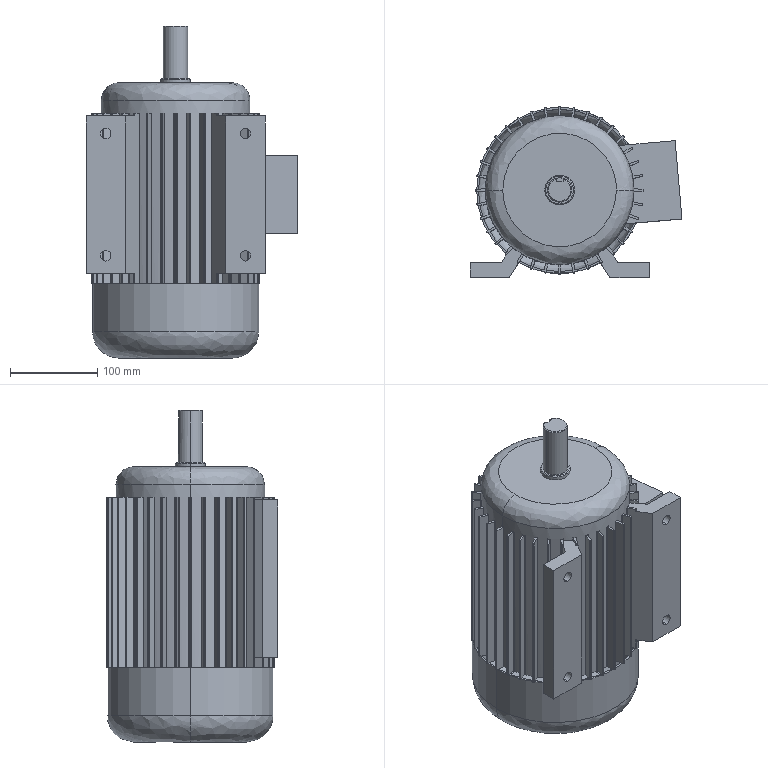Part | SolidWorks | features BaseBody 2 | 2 solids | 448 faces | box 242.5 x 196 x 380 mm | volume 6368698 mm3 | cylinder 285 | plane 152 | spline 6 | cone 5 | commonest cylinder face diameters 1 x215 192 x45 170 x9 12 x8 28 x2 34 x2